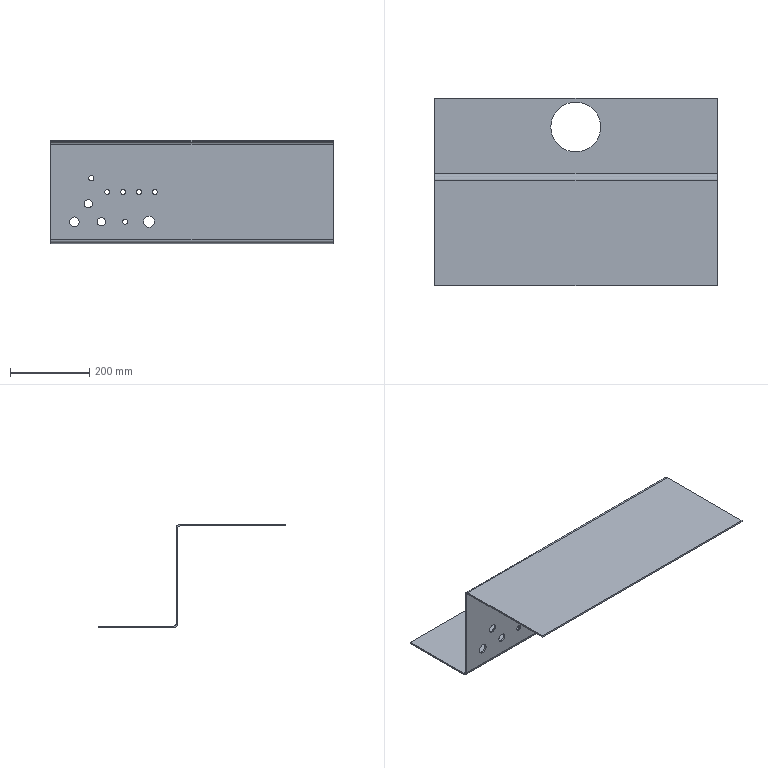Part | SolidWorks | features ICE 2, FlatPattern 1, SMBaseFlange 1, SheetMetal 1 | 1 solid | 44 faces | box 711 x 472 x 260 mm | volume 1991035 mm3 | cylinder 26 | plane 18 | commonest cylinder face diameters 12.5 x10 20.5 x4 12 x2 13.2 x2 20 x2 24.5 x2
STEP:
#1=CARTESIAN_POINT('',(-296.5,-200.,38.75));
#2=VERTEX_POINT('',#1);
#3=CARTESIAN_POINT('',(-296.5,-200.,63.25));
#4=VERTEX_POINT('',#3);
#5=CARTESIAN_POINT('',(-296.5,-200.,51.));
#6=DIRECTION('',(0.,1.,0.));
#7=DIRECTION('',(0.,0.,-1.));
#8=AXIS2_PLACEMENT_3D('',#5,#6,#7);
#9=CIRCLE('',#8,12.25);
#10=EDGE_CURVE('',#2,#4,#9,.T.);
#11=ORIENTED_EDGE('',*,*,#10,.F.);
#12=CARTESIAN_POINT('',(-296.5,-196.,38.75));
#13=VERTEX_POINT('',#12);
#14=CARTESIAN_POINT('',(-296.5,-472.001,38.75));
#15=DIRECTION('',(0.,1.,0.));
#16=VECTOR('',#15,1000.);
#17=LINE('',#14,#16);
#18=EDGE_CURVE('',#2,#13,#17,.T.);
#19=ORIENTED_EDGE('',*,*,#18,.T.);
#20=CARTESIAN_POINT('',(-296.5,-196.,63.25));
#21=VERTEX_POINT('',#20);
#22=CARTESIAN_POINT('',(-296.5,-196.,51.));
#23=DIRECTION('',(0.,1.,0.));
#24=DIRECTION('',(0.,0.,1.));
#25=AXIS2_PLACEMENT_3D('',#22,#23,#24);
#26=CIRCLE('',#25,12.25);
#27=EDGE_CURVE('',#13,#21,#26,.T.);
#28=ORIENTED_EDGE('',*,*,#27,.T.);
#29=CARTESIAN_POINT('',(-296.5,-472.001,63.25));
#30=DIRECTION('',(0.,1.,0.));
#31=VECTOR('',#30,1000.);
#32=LINE('',#29,#31);
#33=EDGE_CURVE('',#4,#21,#32,.T.);
#34=ORIENTED_EDGE('',*,*,#33,.F.);
#35=EDGE_LOOP('',(#11,#19,#28,#34));
#36=FACE_OUTER_BOUND('',#35,.T.);
#37=CARTESIAN_POINT('',(-296.5,-472.001,51.));
#38=DIRECTION('',(0.,1.,0.));
#39=DIRECTION('',(0.,0.,1.));
#40=AXIS2_PLACEMENT_3D('',#37,#38,#39);
#41=CYLINDRICAL_SURFACE('',#40,12.25);
#42=ADVANCED_FACE('',(#36),#41,.F.);
#43=CARTESIAN_POINT('',(-261.5,-200.,85.75));
#44=VERTEX_POINT('',#43);
#45=CARTESIAN_POINT('',(-261.5,-200.,106.25));
#46=VERTEX_POINT('',#45);
#47=CARTESIAN_POINT('',(-261.5,-200.,96.));
#48=DIRECTION('',(0.,1.,0.));
#49=DIRECTION('',(0.,0.,-1.));
#50=AXIS2_PLACEMENT_3D('',#47,#48,#49);
#51=CIRCLE('',#50,10.25);
#52=EDGE_CURVE('',#44,#46,#51,.T.);
#53=ORIENTED_EDGE('',*,*,#52,.F.);
#54=CARTESIAN_POINT('',(-261.5,-196.,85.75));
#55=VERTEX_POINT('',#54);
#56=CARTESIAN_POINT('',(-261.5,-472.001,85.75));
#57=DIRECTION('',(0.,1.,0.));
#58=VECTOR('',#57,1000.);
#59=LINE('',#56,#58);
#60=EDGE_CURVE('',#44,#55,#59,.T.);
#61=ORIENTED_EDGE('',*,*,#60,.T.);
#62=CARTESIAN_POINT('',(-261.5,-196.,106.25));
#63=VERTEX_POINT('',#62);
#64=CARTESIAN_POINT('',(-261.5,-196.,96.));
#65=DIRECTION('',(0.,1.,0.));
#66=DIRECTION('',(0.,0.,1.));
#67=AXIS2_PLACEMENT_3D('',#64,#65,#66);
#68=CIRCLE('',#67,10.25);
#69=EDGE_CURVE('',#55,#63,#68,.T.);
#70=ORIENTED_EDGE('',*,*,#69,.T.);
#71=CARTESIAN_POINT('',(-261.5,-472.001,106.25));
#72=DIRECTION('',(0.,1.,0.));
#73=VECTOR('',#72,1000.);
#74=LINE('',#71,#73);
#75=EDGE_CURVE('',#46,#63,#74,.T.);
#76=ORIENTED_EDGE('',*,*,#75,.F.);
#77=EDGE_LOOP('',(#53,#61,#70,#76));
#78=FACE_OUTER_BOUND('',#77,.T.);
#79=CARTESIAN_POINT('',(-261.5,-472.001,96.));
#80=DIRECTION('',(0.,1.,0.));
#81=DIRECTION('',(0.,0.,1.));
#82=AXIS2_PLACEMENT_3D('',#79,#80,#81);
#83=CYLINDRICAL_SURFACE('',#82,10.25);
#84=ADVANCED_FACE('',(#78),#83,.F.);
#85=CARTESIAN_POINT('',(-108.5,-200.,37.));
#86=VERTEX_POINT('',#85);
#87=CARTESIAN_POINT('',(-108.5,-200.,65.));
#88=VERTEX_POINT('',#87);
#89=CARTESIAN_POINT('',(-108.5,-200.,51.));
#90=DIRECTION('',(0.,1.,0.));
#91=DIRECTION('',(0.,0.,-1.));
#92=AXIS2_PLACEMENT_3D('',#89,#90,#91);
#93=CIRCLE('',#92,14.);
#94=EDGE_CURVE('',#86,#88,#93,.T.);
#95=ORIENTED_EDGE('',*,*,#94,.F.);
#96=CARTESIAN_POINT('',(-108.5,-196.,37.));
#97=VERTEX_POINT('',#96);
#98=CARTESIAN_POINT('',(-108.5,-472.001,37.));
#99=DIRECTION('',(0.,1.,0.));
#100=VECTOR('',#99,1000.);
#101=LINE('',#98,#100);
#102=EDGE_CURVE('',#86,#97,#101,.T.);
#103=ORIENTED_EDGE('',*,*,#102,.T.);
#104=CARTESIAN_POINT('',(-108.5,-196.,65.));
#105=VERTEX_POINT('',#104);
#106=CARTESIAN_POINT('',(-108.5,-196.,51.));
#107=DIRECTION('',(0.,1.,0.));
#108=DIRECTION('',(0.,0.,1.));
#109=AXIS2_PLACEMENT_3D('',#106,#107,#108);
#110=CIRCLE('',#109,14.);
#111=EDGE_CURVE('',#97,#105,#110,.T.);
#112=ORIENTED_EDGE('',*,*,#111,.T.);
#113=CARTESIAN_POINT('',(-108.5,-472.001,65.));
#114=DIRECTION('',(0.,1.,0.));
#115=VECTOR('',#114,1000.);
#116=LINE('',#113,#115);
#117=EDGE_CURVE('',#88,#105,#116,.T.);
#118=ORIENTED_EDGE('',*,*,#117,.F.);
#119=EDGE_LOOP('',(#95,#103,#112,#118));
#120=FACE_OUTER_BOUND('',#119,.T.);
#121=CARTESIAN_POINT('',(-108.5,-472.001,51.));
#122=DIRECTION('',(0.,1.,0.));
#123=DIRECTION('',(0.,0.,1.));
#124=AXIS2_PLACEMENT_3D('',#121,#122,#123);
#125=CYLINDRICAL_SURFACE('',#124,14.);
#126=ADVANCED_FACE('',(#120),#125,.F.);
#127=CARTESIAN_POINT('',(-168.5,-200.,44.75));
#128=VERTEX_POINT('',#127);
#129=CARTESIAN_POINT('',(-168.5,-200.,57.25));
#130=VERTEX_POINT('',#129);
#131=CARTESIAN_POINT('',(-168.5,-200.,51.));
#132=DIRECTION('',(0.,1.,0.));
#133=DIRECTION('',(0.,0.,-1.));
#134=AXIS2_PLACEMENT_3D('',#131,#132,#133);
#135=CIRCLE('',#134,6.25);
#136=EDGE_CURVE('',#128,#130,#135,.T.);
#137=ORIENTED_EDGE('',*,*,#136,.F.);
#138=CARTESIAN_POINT('',(-168.5,-196.,44.75));
#139=VERTEX_POINT('',#138);
#140=CARTESIAN_POINT('',(-168.5,-472.001,44.75));
#141=DIRECTION('',(0.,1.,0.));
#142=VECTOR('',#141,1000.);
#143=LINE('',#140,#142);
#144=EDGE_CURVE('',#128,#139,#143,.T.);
#145=ORIENTED_EDGE('',*,*,#144,.T.);
#146=CARTESIAN_POINT('',(-168.5,-196.,57.25));
#147=VERTEX_POINT('',#146);
#148=CARTESIAN_POINT('',(-168.5,-196.,51.));
#149=DIRECTION('',(0.,1.,0.));
#150=DIRECTION('',(0.,0.,1.));
#151=AXIS2_PLACEMENT_3D('',#148,#149,#150);
#152=CIRCLE('',#151,6.25);
#153=EDGE_CURVE('',#139,#147,#152,.T.);
#154=ORIENTED_EDGE('',*,*,#153,.T.);
#155=CARTESIAN_POINT('',(-168.5,-472.001,57.25));
#156=DIRECTION('',(0.,1.,0.));
#157=VECTOR('',#156,1000.);
#158=LINE('',#155,#157);
#159=EDGE_CURVE('',#130,#147,#158,.T.);
#160=ORIENTED_EDGE('',*,*,#159,.F.);
#161=EDGE_LOOP('',(#137,#145,#154,#160));
#162=FACE_OUTER_BOUND('',#161,.T.);
#163=CARTESIAN_POINT('',(-168.5,-472.001,51.));
#164=DIRECTION('',(0.,1.,0.));
#165=DIRECTION('',(0.,0.,1.));
#166=AXIS2_PLACEMENT_3D('',#163,#164,#165);
#167=CYLINDRICAL_SURFACE('',#166,6.25);
#168=ADVANCED_FACE('',(#162),#167,.F.);
#169=CARTESIAN_POINT('',(-228.5,-200.,40.75));
#170=VERTEX_POINT('',#169);
#171=CARTESIAN_POINT('',(-228.5,-200.,61.25));
#172=VERTEX_POINT('',#171);
#173=CARTESIAN_POINT('',(-228.5,-200.,51.));
#174=DIRECTION('',(0.,1.,0.));
#175=DIRECTION('',(0.,0.,-1.));
#176=AXIS2_PLACEMENT_3D('',#173,#174,#175);
#177=CIRCLE('',#176,10.25);
#178=EDGE_CURVE('',#170,#172,#177,.T.);
#179=ORIENTED_EDGE('',*,*,#178,.F.);
#180=CARTESIAN_POINT('',(-228.5,-196.,40.75));
#181=VERTEX_POINT('',#180);
#182=CARTESIAN_POINT('',(-228.5,-472.001,40.75));
#183=DIRECTION('',(0.,1.,0.));
#184=VECTOR('',#183,1000.);
#185=LINE('',#182,#184);
#186=EDGE_CURVE('',#170,#181,#185,.T.);
#187=ORIENTED_EDGE('',*,*,#186,.T.);
#188=CARTESIAN_POINT('',(-228.5,-196.,61.25));
#189=VERTEX_POINT('',#188);
#190=CARTESIAN_POINT('',(-228.5,-196.,51.));
#191=DIRECTION('',(0.,1.,0.));
#192=DIRECTION('',(0.,0.,1.));
#193=AXIS2_PLACEMENT_3D('',#190,#191,#192);
#194=CIRCLE('',#193,10.25);
#195=EDGE_CURVE('',#181,#189,#194,.T.);
#196=ORIENTED_EDGE('',*,*,#195,.T.);
#197=CARTESIAN_POINT('',(-228.5,-472.001,61.25));
#198=DIRECTION('',(0.,1.,0.));
#199=VECTOR('',#198,1000.);
#200=LINE('',#197,#199);
#201=EDGE_CURVE('',#172,#189,#200,.T.);
#202=ORIENTED_EDGE('',*,*,#201,.F.);
#203=EDGE_LOOP('',(#179,#187,#196,#202));
#204=FACE_OUTER_BOUND('',#203,.T.);
#205=CARTESIAN_POINT('',(-228.5,-472.001,51.));
#206=DIRECTION('',(0.,1.,0.));
#207=DIRECTION('',(0.,0.,1.));
#208=AXIS2_PLACEMENT_3D('',#205,#206,#207);
#209=CYLINDRICAL_SURFACE('',#208,10.25);
#210=ADVANCED_FACE('',(#204),#209,.F.);
#211=CARTESIAN_POINT('',(-213.5,-200.,119.75));
#212=VERTEX_POINT('',#211);
#213=CARTESIAN_POINT('',(-213.5,-200.,132.25));
#214=VERTEX_POINT('',#213);
#215=CARTESIAN_POINT('',(-213.5,-200.,126.));
#216=DIRECTION('',(0.,1.,0.));
#217=DIRECTION('',(0.,0.,-1.));
#218=AXIS2_PLACEMENT_3D('',#215,#216,#217);
#219=CIRCLE('',#218,6.25);
#220=EDGE_CURVE('',#212,#214,#219,.T.);
#221=ORIENTED_EDGE('',*,*,#220,.F.);
#222=CARTESIAN_POINT('',(-213.5,-196.,119.75));
#223=VERTEX_POINT('',#222);
#224=CARTESIAN_POINT('',(-213.5,-472.001,119.75));
#225=DIRECTION('',(0.,1.,0.));
#226=VECTOR('',#225,1000.);
#227=LINE('',#224,#226);
#228=EDGE_CURVE('',#212,#223,#227,.T.);
#229=ORIENTED_EDGE('',*,*,#228,.T.);
#230=CARTESIAN_POINT('',(-213.5,-196.,132.25));
#231=VERTEX_POINT('',#230);
#232=CARTESIAN_POINT('',(-213.5,-196.,126.));
#233=DIRECTION('',(0.,1.,0.));
#234=DIRECTION('',(0.,0.,1.));
#235=AXIS2_PLACEMENT_3D('',#232,#233,#234);
#236=CIRCLE('',#235,6.25);
#237=EDGE_CURVE('',#223,#231,#236,.T.);
#238=ORIENTED_EDGE('',*,*,#237,.T.);
#239=CARTESIAN_POINT('',(-213.5,-472.001,132.25));
#240=DIRECTION('',(0.,1.,0.));
#241=VECTOR('',#240,1000.);
#242=LINE('',#239,#241);
#243=EDGE_CURVE('',#214,#231,#242,.T.);
#244=ORIENTED_EDGE('',*,*,#243,.F.);
#245=EDGE_LOOP('',(#221,#229,#238,#244));
#246=FACE_OUTER_BOUND('',#245,.T.);
#247=CARTESIAN_POINT('',(-213.5,-472.001,126.));
#248=DIRECTION('',(0.,1.,0.));
#249=DIRECTION('',(0.,0.,1.));
#250=AXIS2_PLACEMENT_3D('',#247,#248,#249);
#251=CYLINDRICAL_SURFACE('',#250,6.25);
#252=ADVANCED_FACE('',(#246),#251,.F.);
#253=CARTESIAN_POINT('',(-173.5,-200.,119.75));
#254=VERTEX_POINT('',#253);
#255=CARTESIAN_POINT('',(-173.5,-200.,132.25));
#256=VERTEX_POINT('',#255);
#257=CARTESIAN_POINT('',(-173.5,-200.,126.));
#258=DIRECTION('',(0.,1.,0.));
#259=DIRECTION('',(0.,0.,-1.));
#260=AXIS2_PLACEMENT_3D('',#257,#258,#259);
#261=CIRCLE('',#260,6.25);
#262=EDGE_CURVE('',#254,#256,#261,.T.);
#263=ORIENTED_EDGE('',*,*,#262,.F.);
#264=CARTESIAN_POINT('',(-173.5,-196.,119.75));
#265=VERTEX_POINT('',#264);
#266=CARTESIAN_POINT('',(-173.5,-472.001,119.75));
#267=DIRECTION('',(0.,1.,0.));
#268=VECTOR('',#267,1000.);
#269=LINE('',#266,#268);
#270=EDGE_CURVE('',#254,#265,#269,.T.);
#271=ORIENTED_EDGE('',*,*,#270,.T.);
#272=CARTESIAN_POINT('',(-173.5,-196.,132.25));
#273=VERTEX_POINT('',#272);
#274=CARTESIAN_POINT('',(-173.5,-196.,126.));
#275=DIRECTION('',(0.,1.,0.));
#276=DIRECTION('',(0.,0.,1.));
#277=AXIS2_PLACEMENT_3D('',#274,#275,#276);
#278=CIRCLE('',#277,6.25);
#279=EDGE_CURVE('',#265,#273,#278,.T.);
#280=ORIENTED_EDGE('',*,*,#279,.T.);
#281=CARTESIAN_POINT('',(-173.5,-472.001,132.25));
#282=DIRECTION('',(0.,1.,0.));
#283=VECTOR('',#282,1000.);
#284=LINE('',#281,#283);
#285=EDGE_CURVE('',#256,#273,#284,.T.);
#286=ORIENTED_EDGE('',*,*,#285,.F.);
#287=EDGE_LOOP('',(#263,#271,#280,#286));
#288=FACE_OUTER_BOUND('',#287,.T.);
#289=CARTESIAN_POINT('',(-173.5,-472.001,126.));
#290=DIRECTION('',(0.,1.,0.));
#291=DIRECTION('',(0.,0.,1.));
#292=AXIS2_PLACEMENT_3D('',#289,#290,#291);
#293=CYLINDRICAL_SURFACE('',#292,6.25);
#294=ADVANCED_FACE('',(#288),#293,.F.);
#295=CARTESIAN_POINT('',(-133.5,-200.,119.75));
#296=VERTEX_POINT('',#295);
#297=CARTESIAN_POINT('',(-133.5,-200.,132.25));
#298=VERTEX_POINT('',#297);
#299=CARTESIAN_POINT('',(-133.5,-200.,126.));
#300=DIRECTION('',(0.,1.,0.));
#301=DIRECTION('',(0.,0.,-1.));
#302=AXIS2_PLACEMENT_3D('',#299,#300,#301);
#303=CIRCLE('',#302,6.25);
#304=EDGE_CURVE('',#296,#298,#303,.T.);
#305=ORIENTED_EDGE('',*,*,#304,.F.);
#306=CARTESIAN_POINT('',(-133.5,-196.,119.75));
#307=VERTEX_POINT('',#306);
#308=CARTESIAN_POINT('',(-133.5,-472.001,119.75));
#309=DIRECTION('',(0.,1.,0.));
#310=VECTOR('',#309,1000.);
#311=LINE('',#308,#310);
#312=EDGE_CURVE('',#296,#307,#311,.T.);
#313=ORIENTED_EDGE('',*,*,#312,.T.);
#314=CARTESIAN_POINT('',(-133.5,-196.,132.25));
#315=VERTEX_POINT('',#314);
#316=CARTESIAN_POINT('',(-133.5,-196.,126.));
#317=DIRECTION('',(0.,1.,0.));
#318=DIRECTION('',(0.,0.,1.));
#319=AXIS2_PLACEMENT_3D('',#316,#317,#318);
#320=CIRCLE('',#319,6.25);
#321=EDGE_CURVE('',#307,#315,#320,.T.);
#322=ORIENTED_EDGE('',*,*,#321,.T.);
#323=CARTESIAN_POINT('',(-133.5,-472.001,132.25));
#324=DIRECTION('',(0.,1.,0.));
#325=VECTOR('',#324,1000.);
#326=LINE('',#323,#325);
#327=EDGE_CURVE('',#298,#315,#326,.T.);
#328=ORIENTED_EDGE('',*,*,#327,.F.);
#329=EDGE_LOOP('',(#305,#313,#322,#328));
#330=FACE_OUTER_BOUND('',#329,.T.);
#331=CARTESIAN_POINT('',(-133.5,-472.001,126.));
#332=DIRECTION('',(0.,1.,0.));
#333=DIRECTION('',(0.,0.,1.));
#334=AXIS2_PLACEMENT_3D('',#331,#332,#333);
#335=CYLINDRICAL_SURFACE('',#334,6.25);
#336=ADVANCED_FACE('',(#330),#335,.F.);
#337=CARTESIAN_POINT('',(-93.5,-200.,119.75));
#338=VERTEX_POINT('',#337);
#339=CARTESIAN_POINT('',(-93.5,-200.,132.25));
#340=VERTEX_POINT('',#339);
#341=CARTESIAN_POINT('',(-93.5,-200.,126.));
#342=DIRECTION('',(0.,1.,0.));
#343=DIRECTION('',(0.,0.,-1.));
#344=AXIS2_PLACEMENT_3D('',#341,#342,#343);
#345=CIRCLE('',#344,6.25);
#346=EDGE_CURVE('',#338,#340,#345,.T.);
#347=ORIENTED_EDGE('',*,*,#346,.F.);
#348=CARTESIAN_POINT('',(-93.5,-196.,119.75));
#349=VERTEX_POINT('',#348);
#350=CARTESIAN_POINT('',(-93.5,-472.001,119.75));
#351=DIRECTION('',(0.,1.,0.));
#352=VECTOR('',#351,1000.);
#353=LINE('',#350,#352);
#354=EDGE_CURVE('',#338,#349,#353,.T.);
#355=ORIENTED_EDGE('',*,*,#354,.T.);
#356=CARTESIAN_POINT('',(-93.5,-196.,132.25));
#357=VERTEX_POINT('',#356);
#358=CARTESIAN_POINT('',(-93.5,-196.,126.));
#359=DIRECTION('',(0.,1.,0.));
#360=DIRECTION('',(0.,0.,1.));
#361=AXIS2_PLACEMENT_3D('',#358,#359,#360);
#362=CIRCLE('',#361,6.25);
#363=EDGE_CURVE('',#349,#357,#362,.T.);
#364=ORIENTED_EDGE('',*,*,#363,.T.);
#365=CARTESIAN_POINT('',(-93.5,-472.001,132.25));
#366=DIRECTION('',(0.,1.,0.));
#367=VECTOR('',#366,1000.);
#368=LINE('',#365,#367);
#369=EDGE_CURVE('',#340,#357,#368,.T.);
#370=ORIENTED_EDGE('',*,*,#369,.F.);
#371=EDGE_LOOP('',(#347,#355,#364,#370));
#372=FACE_OUTER_BOUND('',#371,.T.);
#373=CARTESIAN_POINT('',(-93.5,-472.001,126.));
#374=DIRECTION('',(0.,1.,0.));
#375=DIRECTION('',(0.,0.,1.));
#376=AXIS2_PLACEMENT_3D('',#373,#374,#375);
#377=CYLINDRICAL_SURFACE('',#376,6.25);
#378=ADVANCED_FACE('',(#372),#377,.F.);
#379=CARTESIAN_POINT('',(-253.5,-200.,154.4));
#380=VERTEX_POINT('',#379);
#381=CARTESIAN_POINT('',(-253.5,-200.,167.6));
#382=VERTEX_POINT('',#381);
#383=CARTESIAN_POINT('',(-253.5,-200.,161.));
#384=DIRECTION('',(0.,1.,0.));
#385=DIRECTION('',(0.,0.,-1.));
#386=AXIS2_PLACEMENT_3D('',#383,#384,#385);
#387=CIRCLE('',#386,6.6);
#388=EDGE_CURVE('',#380,#382,#387,.T.);
#389=ORIENTED_EDGE('',*,*,#388,.F.);
#390=CARTESIAN_POINT('',(-253.5,-196.,154.4));
#391=VERTEX_POINT('',#390);
#392=CARTESIAN_POINT('',(-253.5,-472.001,154.4));
#393=DIRECTION('',(0.,1.,0.));
#394=VECTOR('',#393,1000.);
#395=LINE('',#392,#394);
#396=EDGE_CURVE('',#380,#391,#395,.T.);
#397=ORIENTED_EDGE('',*,*,#396,.T.);
#398=CARTESIAN_POINT('',(-253.5,-196.,167.6));
#399=VERTEX_POINT('',#398);
#400=CARTESIAN_POINT('',(-253.5,-196.,161.));
#401=DIRECTION('',(0.,1.,0.));
#402=DIRECTION('',(0.,0.,1.));
#403=AXIS2_PLACEMENT_3D('',#400,#401,#402);
#404=CIRCLE('',#403,6.6);
#405=EDGE_CURVE('',#391,#399,#404,.T.);
#406=ORIENTED_EDGE('',*,*,#405,.T.);
#407=CARTESIAN_POINT('',(-253.5,-472.001,167.6));
#408=DIRECTION('',(0.,1.,0.));
#409=VECTOR('',#408,1000.);
#410=LINE('',#407,#409);
#411=EDGE_CURVE('',#382,#399,#410,.T.);
#412=ORIENTED_EDGE('',*,*,#411,.F.);
#413=EDGE_LOOP('',(#389,#397,#406,#412));
#414=FACE_OUTER_BOUND('',#413,.T.);
#415=CARTESIAN_POINT('',(-253.5,-472.001,161.));
#416=DIRECTION('',(0.,1.,0.));
#417=DIRECTION('',(0.,0.,1.));
#418=AXIS2_PLACEMENT_3D('',#415,#416,#417);
#419=CYLINDRICAL_SURFACE('',#418,6.6);
#420=ADVANCED_FACE('',(#414),#419,.F.);
#421=CARTESIAN_POINT('',(-63.7,-72.,0.));
#422=VERTEX_POINT('',#421);
#423=CARTESIAN_POINT('',(62.3,-72.,0.));
#424=VERTEX_POINT('',#423);
#425=CARTESIAN_POINT('',(-0.7,-72.,0.));
#426=DIRECTION('',(0.,0.,1.));
#427=DIRECTION('',(-1.,0.,0.));
#428=AXIS2_PLACEMENT_3D('',#425,#426,#427);
#429=CIRCLE('',#428,63.);
#430=EDGE_CURVE('',#422,#424,#429,.T.);
#431=ORIENTED_EDGE('',*,*,#430,.T.);
#432=CARTESIAN_POINT('',(62.3,-72.,-4.));
#433=VERTEX_POINT('',#432);
#434=CARTESIAN_POINT('',(62.3,-72.,256.001));
#435=DIRECTION('',(0.,0.,-1.));
#436=VECTOR('',#435,1000.);
#437=LINE('',#434,#436);
#438=EDGE_CURVE('',#424,#433,#437,.T.);
#439=ORIENTED_EDGE('',*,*,#438,.T.);
#440=CARTESIAN_POINT('',(-63.7,-72.,-4.));
#441=VERTEX_POINT('',#440);
#442=CARTESIAN_POINT('',(-0.7,-72.,-4.));
#443=DIRECTION('',(0.,0.,-1.));
#444=DIRECTION('',(-1.,0.,0.));
#445=AXIS2_PLACEMENT_3D('',#442,#443,#444);
#446=CIRCLE('',#445,63.);
#447=EDGE_CURVE('',#433,#441,#446,.T.);
#448=ORIENTED_EDGE('',*,*,#447,.T.);
#449=CARTESIAN_POINT('',(-63.7,-72.,256.001));
#450=DIRECTION('',(0.,0.,-1.));
#451=VECTOR('',#450,1000.);
#452=LINE('',#449,#451);
#453=EDGE_CURVE('',#422,#441,#452,.T.);
#454=ORIENTED_EDGE('',*,*,#453,.F.);
#455=EDGE_LOOP('',(#431,#439,#448,#454));
#456=FACE_OUTER_BOUND('',#455,.T.);
#457=CARTESIAN_POINT('',(-0.7,-72.,256.001));
#458=DIRECTION('',(0.,0.,-1.));
#459=DIRECTION('',(-1.,0.,0.));
#460=AXIS2_PLACEMENT_3D('',#457,#458,#459);
#461=CYLINDRICAL_SURFACE('',#460,63.);
#462=ADVANCED_FACE('',(#456),#461,.F.);
#463=CARTESIAN_POINT('',(355.5,-190.,0.));
#464=VERTEX_POINT('',#463);
#465=CARTESIAN_POINT('',(355.5,-190.,-4.));
#466=VERTEX_POINT('',#465);
#467=CARTESIAN_POINT('',(355.5,-190.,0.));
#468=DIRECTION('',(0.,0.,-1.));
#469=VECTOR('',#468,1000.);
#470=LINE('',#467,#469);
#471=EDGE_CURVE('',#464,#466,#470,.T.);
#472=ORIENTED_EDGE('',*,*,#471,.F.);
#473=CARTESIAN_POINT('',(355.5,-196.,6.));
#474=VERTEX_POINT('',#473);
#475=CARTESIAN_POINT('',(355.5,-190.,6.));
#476=DIRECTION('',(-1.,0.,0.));
#477=DIRECTION('',(0.,0.,-1.));
#478=AXIS2_PLACEMENT_3D('',#475,#476,#477);
#479=CIRCLE('',#478,6.);
#480=EDGE_CURVE('',#464,#474,#479,.T.);
#481=ORIENTED_EDGE('',*,*,#480,.T.);
#482=CARTESIAN_POINT('',(355.5,-200.,6.));
#483=VERTEX_POINT('',#482);
#484=CARTESIAN_POINT('',(355.5,-200.,6.));
#485=DIRECTION('',(0.,1.,0.));
#486=VECTOR('',#485,1000.);
#487=LINE('',#484,#486);
#488=EDGE_CURVE('',#483,#474,#487,.T.);
#489=ORIENTED_EDGE('',*,*,#488,.F.);
#490=CARTESIAN_POINT('',(355.5,-190.,6.));
#491=DIRECTION('',(-1.,0.,0.));
#492=DIRECTION('',(0.,0.,-1.));
#493=AXIS2_PLACEMENT_3D('',#490,#491,#492);
#494=CIRCLE('',#493,10.);
#495=EDGE_CURVE('',#466,#483,#494,.T.);
#496=ORIENTED_EDGE('',*,*,#495,.F.);
#497=EDGE_LOOP('',(#472,#481,#489,#496));
#498=FACE_OUTER_BOUND('',#497,.T.);
#499=CARTESIAN_POINT('',(355.5,-190.,0.));
#500=DIRECTION('',(1.,0.,0.));
#501=DIRECTION('',(0.,0.,-1.));
#502=AXIS2_PLACEMENT_3D('',#499,#500,#501);
#503=PLANE('',#502);
#504=ADVANCED_FACE('',(#498),#503,.T.);
#505=CARTESIAN_POINT('',(355.5,0.,0.));
#506=VERTEX_POINT('',#505);
#507=CARTESIAN_POINT('',(355.5,0.,0.));
#508=DIRECTION('',(0.,-1.,0.));
#509=VECTOR('',#508,1000.);
#510=LINE('',#507,#509);
#511=EDGE_CURVE('',#506,#464,#510,.T.);
#512=ORIENTED_EDGE('',*,*,#511,.T.);
#513=ORIENTED_EDGE('',*,*,#471,.T.);
#514=CARTESIAN_POINT('',(355.5,0.,-4.));
#515=VERTEX_POINT('',#514);
#516=CARTESIAN_POINT('',(355.5,0.,-4.));
#517=DIRECTION('',(0.,-1.,0.));
#518=VECTOR('',#517,1000.);
#519=LINE('',#516,#518);
#520=EDGE_CURVE('',#515,#466,#519,.T.);
#521=ORIENTED_EDGE('',*,*,#520,.F.);
#522=CARTESIAN_POINT('',(355.5,0.,0.));
#523=DIRECTION('',(0.,0.,-1.));
#524=VECTOR('',#523,1000.);
#525=LINE('',#522,#524);
#526=EDGE_CURVE('',#506,#515,#525,.T.);
#527=ORIENTED_EDGE('',*,*,#526,.F.);
#528=EDGE_LOOP('',(#512,#513,#521,#527));
#529=FACE_OUTER_BOUND('',#528,.T.);
#530=CARTESIAN_POINT('',(355.5,-200.,6.));
#531=DIRECTION('',(1.,0.,0.));
#532=DIRECTION('',(0.,0.,-1.));
#533=AXIS2_PLACEMENT_3D('',#530,#531,#532);
#534=PLANE('',#533);
#535=ADVANCED_FACE('',(#529),#534,.T.);
#536=CARTESIAN_POINT('',(-355.5,-196.,6.));
#537=VERTEX_POINT('',#536);
#538=CARTESIAN_POINT('',(-355.5,-200.,6.));
#539=VERTEX_POINT('',#538);
#540=CARTESIAN_POINT('',(-355.5,-196.,6.));
#541=DIRECTION('',(0.,-1.,0.));
#542=VECTOR('',#541,1000.);
#543=LINE('',#540,#542);
#544=EDGE_CURVE('',#537,#539,#543,.T.);
#545=ORIENTED_EDGE('',*,*,#544,.F.);
#546=CARTESIAN_POINT('',(-355.5,-190.,0.));
#547=VERTEX_POINT('',#546);
#548=CARTESIAN_POINT('',(-355.5,-190.,6.));
#549=DIRECTION('',(-1.,0.,0.));
#550=DIRECTION('',(0.,0.,-1.));
#551=AXIS2_PLACEMENT_3D('',#548,#549,#550);
#552=CIRCLE('',#551,6.);
#553=EDGE_CURVE('',#547,#537,#552,.T.);
#554=ORIENTED_EDGE('',*,*,#553,.F.);
#555=CARTESIAN_POINT('',(-355.5,-190.,-4.));
#556=VERTEX_POINT('',#555);
#557=CARTESIAN_POINT('',(-355.5,-190.,-4.));
#558=DIRECTION('',(0.,0.,1.));
#559=VECTOR('',#558,1000.);
#560=LINE('',#557,#559);
#561=EDGE_CURVE('',#556,#547,#560,.T.);
#562=ORIENTED_EDGE('',*,*,#561,.F.);
#563=CARTESIAN_POINT('',(-355.5,-190.,6.));
#564=DIRECTION('',(-1.,0.,0.));
#565=DIRECTION('',(0.,0.,-1.));
#566=AXIS2_PLACEMENT_3D('',#563,#564,#565);
#567=CIRCLE('',#566,10.);
#568=EDGE_CURVE('',#556,#539,#567,.T.);
#569=ORIENTED_EDGE('',*,*,#568,.T.);
#570=EDGE_LOOP('',(#545,#554,#562,#569));
#571=FACE_OUTER_BOUND('',#570,.T.);
#572=CARTESIAN_POINT('',(-355.5,-196.,6.));
#573=DIRECTION('',(-1.,0.,0.));
#574=DIRECTION('',(0.,0.,1.));
#575=AXIS2_PLACEMENT_3D('',#572,#573,#574);
#576=PLANE('',#575);
#577=ADVANCED_FACE('',(#571),#576,.T.);
#578=CARTESIAN_POINT('',(-355.5,-196.,246.));
#579=VERTEX_POINT('',#578);
#580=CARTESIAN_POINT('',(-355.5,-196.,0.));
#581=DIRECTION('',(0.,0.,1.));
#582=VECTOR('',#581,1000.);
#583=LINE('',#580,#582);
#584=EDGE_CURVE('',#537,#579,#583,.T.);
#585=ORIENTED_EDGE('',*,*,#584,.F.);
#586=ORIENTED_EDGE('',*,*,#544,.T.);
#587=CARTESIAN_POINT('',(-355.5,-200.,246.));
#588=VERTEX_POINT('',#587);
#589=CARTESIAN_POINT('',(-355.5,-200.,0.));
#590=DIRECTION('',(0.,0.,1.));
#591=VECTOR('',#590,1000.);
#592=LINE('',#589,#591);
#593=EDGE_CURVE('',#539,#588,#592,.T.);
#594=ORIENTED_EDGE('',*,*,#593,.T.);
#595=CARTESIAN_POINT('',(-355.5,-200.,246.));
#596=DIRECTION('',(0.,1.,0.));
#597=VECTOR('',#596,1000.);
#598=LINE('',#595,#597);
#599=EDGE_CURVE('',#588,#579,#598,.T.);
#600=ORIENTED_EDGE('',*,*,#599,.T.);
#601=EDGE_LOOP('',(#585,#586,#594,#600));
#602=FACE_OUTER_BOUND('',#601,.T.);
#603=CARTESIAN_POINT('',(-355.5,-190.,-4.));
#604=DIRECTION('',(-1.,0.,0.));
#605=DIRECTION('',(0.,0.,1.));
#606=AXIS2_PLACEMENT_3D('',#603,#604,#605);
#607=PLANE('',#606);
#608=ADVANCED_FACE('',(#602),#607,.T.);
#609=CARTESIAN_POINT('',(355.5,-196.,246.));
#610=VERTEX_POINT('',#609);
#611=CARTESIAN_POINT('',(355.5,-200.,246.));
#612=VERTEX_POINT('',#611);
#613=CARTESIAN_POINT('',(355.5,-196.,246.));
#614=DIRECTION('',(0.,-1.,0.));
#615=VECTOR('',#614,1000.);
#616=LINE('',#613,#615);
#617=EDGE_CURVE('',#610,#612,#616,.T.);
#618=ORIENTED_EDGE('',*,*,#617,.F.);
#619=CARTESIAN_POINT('',(355.5,-206.,256.));
#620=VERTEX_POINT('',#619);
#621=CARTESIAN_POINT('',(355.5,-206.,246.));
#622=DIRECTION('',(1.,0.,0.));
#623=DIRECTION('',(0.,0.,1.));
#624=AXIS2_PLACEMENT_3D('',#621,#622,#623);
#625=CIRCLE('',#624,10.);
#626=EDGE_CURVE('',#610,#620,#625,.T.);
#627=ORIENTED_EDGE('',*,*,#626,.T.);
#628=CARTESIAN_POINT('',(355.5,-206.,252.));
#629=VERTEX_POINT('',#628);
#630=CARTESIAN_POINT('',(355.5,-206.,252.));
#631=DIRECTION('',(0.,0.,1.));
#632=VECTOR('',#631,1000.);
#633=LINE('',#630,#632);
#634=EDGE_CURVE('',#629,#620,#633,.T.);
#635=ORIENTED_EDGE('',*,*,#634,.F.);
#636=CARTESIAN_POINT('',(355.5,-206.,246.));
#637=DIRECTION('',(1.,0.,0.));
#638=DIRECTION('',(0.,0.,-1.));
#639=AXIS2_PLACEMENT_3D('',#636,#637,#638);
#640=CIRCLE('',#639,6.);
#641=EDGE_CURVE('',#612,#629,#640,.T.);
#642=ORIENTED_EDGE('',*,*,#641,.F.);
#643=EDGE_LOOP('',(#618,#627,#635,#642));
#644=FACE_OUTER_BOUND('',#643,.T.);
#645=CARTESIAN_POINT('',(355.5,-196.,246.));
#646=DIRECTION('',(1.,0.,0.));
#647=DIRECTION('',(0.,0.,-1.));
#648=AXIS2_PLACEMENT_3D('',#645,#646,#647);
#649=PLANE('',#648);
#650=ADVANCED_FACE('',(#644),#649,.T.);
#651=CARTESIAN_POINT('',(355.5,-196.,0.));
#652=DIRECTION('',(0.,0.,1.));
#653=VECTOR('',#652,1000.);
#654=LINE('',#651,#653);
#655=EDGE_CURVE('',#474,#610,#654,.T.);
#656=ORIENTED_EDGE('',*,*,#655,.T.);
#657=ORIENTED_EDGE('',*,*,#617,.T.);
#658=CARTESIAN_POINT('',(355.5,-200.,0.));
#659=DIRECTION('',(0.,0.,1.));
#660=VECTOR('',#659,1000.);
#661=LINE('',#658,#660);
#662=EDGE_CURVE('',#483,#612,#661,.T.);
#663=ORIENTED_EDGE('',*,*,#662,.F.);
#664=ORIENTED_EDGE('',*,*,#488,.T.);
#665=EDGE_LOOP('',(#656,#657,#663,#664));
#666=FACE_OUTER_BOUND('',#665,.T.);
#667=CARTESIAN_POINT('',(355.5,-206.,252.));
#668=DIRECTION('',(1.,0.,0.));
#669=DIRECTION('',(0.,0.,-1.));
#670=AXIS2_PLACEMENT_3D('',#667,#668,#669);
#671=PLANE('',#670);
#672=ADVANCED_FACE('',(#666),#671,.T.);
#673=CARTESIAN_POINT('',(-355.5,-206.,256.));
#674=VERTEX_POINT('',#673);
#675=CARTESIAN_POINT('',(-355.5,-206.,252.));
#676=VERTEX_POINT('',#675);
#677=CARTESIAN_POINT('',(-355.5,-206.,256.));
#678=DIRECTION('',(0.,0.,-1.));
#679=VECTOR('',#678,1000.);
#680=LINE('',#677,#679);
#681=EDGE_CURVE('',#674,#676,#680,.T.);
#682=ORIENTED_EDGE('',*,*,#681,.F.);
#683=CARTESIAN_POINT('',(-355.5,-206.,246.));
#684=DIRECTION('',(1.,0.,0.));
#685=DIRECTION('',(0.,0.,1.));
#686=AXIS2_PLACEMENT_3D('',#683,#684,#685);
#687=CIRCLE('',#686,10.);
#688=EDGE_CURVE('',#579,#674,#687,.T.);
#689=ORIENTED_EDGE('',*,*,#688,.F.);
#690=ORIENTED_EDGE('',*,*,#599,.F.);
#691=CARTESIAN_POINT('',(-355.5,-206.,246.));
#692=DIRECTION('',(1.,0.,0.));
#693=DIRECTION('',(0.,0.,-1.));
#694=AXIS2_PLACEMENT_3D('',#691,#692,#693);
#695=CIRCLE('',#694,6.);
#696=EDGE_CURVE('',#588,#676,#695,.T.);
#697=ORIENTED_EDGE('',*,*,#696,.T.);
#698=EDGE_LOOP('',(#682,#689,#690,#697));
#699=FACE_OUTER_BOUND('',#698,.T.);
#700=CARTESIAN_POINT('',(-355.5,-206.,256.));
#701=DIRECTION('',(-1.,0.,0.));
#702=DIRECTION('',(0.,0.,1.));
#703=AXIS2_PLACEMENT_3D('',#700,#701,#702);
#704=PLANE('',#703);
#705=ADVANCED_FACE('',(#699),#704,.T.);
#706=CARTESIAN_POINT('',(-355.5,-472.,256.));
#707=VERTEX_POINT('',#706);
#708=CARTESIAN_POINT('',(-355.5,-196.,256.));
#709=DIRECTION('',(0.,-1.,0.));
#710=VECTOR('',#709,1000.);
#711=LINE('',#708,#710);
#712=EDGE_CURVE('',#674,#707,#711,.T.);
#713=ORIENTED_EDGE('',*,*,#712,.F.);
#714=ORIENTED_EDGE('',*,*,#681,.T.);
#715=CARTESIAN_POINT('',(-355.5,-472.,252.));
#716=VERTEX_POINT('',#715);
#717=CARTESIAN_POINT('',(-355.5,-196.,252.));
#718=DIRECTION('',(0.,-1.,0.));
#719=VECTOR('',#718,1000.);
#720=LINE('',#717,#719);
#721=EDGE_CURVE('',#676,#716,#720,.T.);
#722=ORIENTED_EDGE('',*,*,#721,.T.);
#723=CARTESIAN_POINT('',(-355.5,-472.,252.));
#724=DIRECTION('',(0.,0.,1.));
#725=VECTOR('',#724,1000.);
#726=LINE('',#723,#725);
#727=EDGE_CURVE('',#716,#707,#726,.T.);
#728=ORIENTED_EDGE('',*,*,#727,.T.);
#729=EDGE_LOOP('',(#713,#714,#722,#728));
#730=FACE_OUTER_BOUND('',#729,.T.);
#731=CARTESIAN_POINT('',(-355.5,-200.,246.));
#732=DIRECTION('',(-1.,0.,0.));
#733=DIRECTION('',(0.,0.,1.));
#734=AXIS2_PLACEMENT_3D('',#731,#732,#733);
#735=PLANE('',#734);
#736=ADVANCED_FACE('',(#730),#735,.T.);
#737=ORIENTED_EDGE('',*,*,#712,.T.);
#738=CARTESIAN_POINT('',(355.5,-472.,256.));
#739=VERTEX_POINT('',#738);
#740=CARTESIAN_POINT('',(355.5,-472.,256.));
#741=DIRECTION('',(-1.,0.,0.));
#742=VECTOR('',#741,1000.);
#743=LINE('',#740,#742);
#744=EDGE_CURVE('',#739,#707,#743,.T.);
#745=ORIENTED_EDGE('',*,*,#744,.F.);
#746=CARTESIAN_POINT('',(355.5,-196.,256.));
#747=DIRECTION('',(0.,-1.,0.));
#748=VECTOR('',#747,1000.);
#749=LINE('',#746,#748);
#750=EDGE_CURVE('',#620,#739,#749,.T.);
#751=ORIENTED_EDGE('',*,*,#750,.F.);
#752=CARTESIAN_POINT('',(355.5,-206.,256.));
#753=DIRECTION('',(-1.,0.,0.));
#754=VECTOR('',#753,1000.);
#755=LINE('',#752,#754);
#756=EDGE_CURVE('',#620,#674,#755,.T.);
#757=ORIENTED_EDGE('',*,*,#756,.T.);
#758=EDGE_LOOP('',(#737,#745,#751,#757));
#759=FACE_OUTER_BOUND('',#758,.T.);
#760=CARTESIAN_POINT('',(355.5,-196.,256.));
#761=DIRECTION('',(0.,0.,-1.));
#762=DIRECTION('',(0.,1.,0.));
#763=AXIS2_PLACEMENT_3D('',#760,#761,#762);
#764=PLANE('',#763);
#765=ADVANCED_FACE('',(#759),#764,.F.);
#766=ORIENTED_EDGE('',*,*,#727,.F.);
#767=CARTESIAN_POINT('',(355.5,-472.,252.));
#768=VERTEX_POINT('',#767);
#769=CARTESIAN_POINT('',(355.5,-472.,252.));
#770=DIRECTION('',(-1.,0.,0.));
#771=VECTOR('',#770,1000.);
#772=LINE('',#769,#771);
#773=EDGE_CURVE('',#768,#716,#772,.T.);
#774=ORIENTED_EDGE('',*,*,#773,.F.);
#775=CARTESIAN_POINT('',(355.5,-472.,252.));
#776=DIRECTION('',(0.,0.,1.));
#777=VECTOR('',#776,1000.);
#778=LINE('',#775,#777);
#779=EDGE_CURVE('',#768,#739,#778,.T.);
#780=ORIENTED_EDGE('',*,*,#779,.T.);
#781=ORIENTED_EDGE('',*,*,#744,.T.);
#782=EDGE_LOOP('',(#766,#774,#780,#781));
#783=FACE_OUTER_BOUND('',#782,.T.);
#784=CARTESIAN_POINT('',(355.5,-472.,252.));
#785=DIRECTION('',(0.,-1.,0.));
#786=DIRECTION('',(0.,0.,-1.));
#787=AXIS2_PLACEMENT_3D('',#784,#785,#786);
#788=PLANE('',#787);
#789=ADVANCED_FACE('',(#783),#788,.T.);
#790=ORIENTED_EDGE('',*,*,#721,.F.);
#791=CARTESIAN_POINT('',(355.5,-206.,252.));
#792=DIRECTION('',(-1.,0.,0.));
#793=VECTOR('',#792,1000.);
#794=LINE('',#791,#793);
#795=EDGE_CURVE('',#629,#676,#794,.T.);
#796=ORIENTED_EDGE('',*,*,#795,.F.);
#797=CARTESIAN_POINT('',(355.5,-196.,252.));
#798=DIRECTION('',(0.,-1.,0.));
#799=VECTOR('',#798,1000.);
#800=LINE('',#797,#799);
#801=EDGE_CURVE('',#629,#768,#800,.T.);
#802=ORIENTED_EDGE('',*,*,#801,.T.);
#803=ORIENTED_EDGE('',*,*,#773,.T.);
#804=EDGE_LOOP('',(#790,#796,#802,#803));
#805=FACE_OUTER_BOUND('',#804,.T.);
#806=CARTESIAN_POINT('',(355.5,-196.,252.));
#807=DIRECTION('',(0.,0.,-1.));
#808=DIRECTION('',(0.,1.,0.));
#809=AXIS2_PLACEMENT_3D('',#806,#807,#808);
#810=PLANE('',#809);
#811=ADVANCED_FACE('',(#805),#810,.T.);
#812=ORIENTED_EDGE('',*,*,#696,.F.);
#813=CARTESIAN_POINT('',(355.5,-200.,246.));
#814=DIRECTION('',(-1.,0.,0.));
#815=VECTOR('',#814,1000.);
#816=LINE('',#813,#815);
#817=EDGE_CURVE('',#612,#588,#816,.T.);
#818=ORIENTED_EDGE('',*,*,#817,.F.);
#819=ORIENTED_EDGE('',*,*,#641,.T.);
#820=ORIENTED_EDGE('',*,*,#795,.T.);
#821=EDGE_LOOP('',(#812,#818,#819,#820));
#822=FACE_OUTER_BOUND('',#821,.T.);
#823=CARTESIAN_POINT('',(355.5,-206.,246.));
#824=DIRECTION('',(-1.,0.,0.));
#825=DIRECTION('',(0.,0.,1.));
#826=AXIS2_PLACEMENT_3D('',#823,#824,#825);
#827=CYLINDRICAL_SURFACE('',#826,6.);
#828=ADVANCED_FACE('',(#822),#827,.F.);
#829=CARTESIAN_POINT('',(-296.5,-200.,51.));
#830=DIRECTION('',(0.,1.,0.));
#831=DIRECTION('',(0.,0.,-1.));
#832=AXIS2_PLACEMENT_3D('',#829,#830,#831);
#833=CIRCLE('',#832,12.25);
#834=EDGE_CURVE('',#4,#2,#833,.T.);
#835=ORIENTED_EDGE('',*,*,#834,.T.);
#836=ORIENTED_EDGE('',*,*,#10,.T.);
#837=EDGE_LOOP('',(#835,#836));
#838=FACE_BOUND('',#837,.T.);
#839=CARTESIAN_POINT('',(-261.5,-200.,96.));
#840=DIRECTION('',(0.,1.,0.));
#841=DIRECTION('',(0.,0.,-1.));
#842=AXIS2_PLACEMENT_3D('',#839,#840,#841);
#843=CIRCLE('',#842,10.25);
#844=EDGE_CURVE('',#46,#44,#843,.T.);
#845=ORIENTED_EDGE('',*,*,#844,.T.);
#846=ORIENTED_EDGE('',*,*,#52,.T.);
#847=EDGE_LOOP('',(#845,#846));
#848=FACE_BOUND('',#847,.T.);
#849=CARTESIAN_POINT('',(-108.5,-200.,51.));
#850=DIRECTION('',(0.,1.,0.));
#851=DIRECTION('',(0.,0.,-1.));
#852=AXIS2_PLACEMENT_3D('',#849,#850,#851);
#853=CIRCLE('',#852,14.);
#854=EDGE_CURVE('',#88,#86,#853,.T.);
#855=ORIENTED_EDGE('',*,*,#854,.T.);
#856=ORIENTED_EDGE('',*,*,#94,.T.);
#857=EDGE_LOOP('',(#855,#856));
#858=FACE_BOUND('',#857,.T.);
#859=CARTESIAN_POINT('',(-168.5,-200.,51.));
#860=DIRECTION('',(0.,1.,0.));
#861=DIRECTION('',(0.,0.,-1.));
#862=AXIS2_PLACEMENT_3D('',#859,#860,#861);
#863=CIRCLE('',#862,6.25);
#864=EDGE_CURVE('',#130,#128,#863,.T.);
#865=ORIENTED_EDGE('',*,*,#864,.T.);
#866=ORIENTED_EDGE('',*,*,#136,.T.);
#867=EDGE_LOOP('',(#865,#866));
#868=FACE_BOUND('',#867,.T.);
#869=CARTESIAN_POINT('',(-228.5,-200.,51.));
#870=DIRECTION('',(0.,1.,0.));
#871=DIRECTION('',(0.,0.,-1.));
#872=AXIS2_PLACEMENT_3D('',#869,#870,#871);
#873=CIRCLE('',#872,10.25);
#874=EDGE_CURVE('',#172,#170,#873,.T.);
#875=ORIENTED_EDGE('',*,*,#874,.T.);
#876=ORIENTED_EDGE('',*,*,#178,.T.);
#877=EDGE_LOOP('',(#875,#876));
#878=FACE_BOUND('',#877,.T.);
#879=CARTESIAN_POINT('',(-213.5,-200.,126.));
#880=DIRECTION('',(0.,1.,0.));
#881=DIRECTION('',(0.,0.,-1.));
#882=AXIS2_PLACEMENT_3D('',#879,#880,#881);
#883=CIRCLE('',#882,6.25);
#884=EDGE_CURVE('',#214,#212,#883,.T.);
#885=ORIENTED_EDGE('',*,*,#884,.T.);
#886=ORIENTED_EDGE('',*,*,#220,.T.);
#887=EDGE_LOOP('',(#885,#886));
#888=FACE_BOUND('',#887,.T.);
#889=CARTESIAN_POINT('',(-173.5,-200.,126.));
#890=DIRECTION('',(0.,1.,0.));
#891=DIRECTION('',(0.,0.,-1.));
#892=AXIS2_PLACEMENT_3D('',#889,#890,#891);
#893=CIRCLE('',#892,6.25);
#894=EDGE_CURVE('',#256,#254,#893,.T.);
#895=ORIENTED_EDGE('',*,*,#894,.T.);
#896=ORIENTED_EDGE('',*,*,#262,.T.);
#897=EDGE_LOOP('',(#895,#896));
#898=FACE_BOUND('',#897,.T.);
#899=CARTESIAN_POINT('',(-133.5,-200.,126.));
#900=DIRECTION('',(0.,1.,0.));
#901=DIRECTION('',(0.,0.,-1.));
#902=AXIS2_PLACEMENT_3D('',#899,#900,#901);
#903=CIRCLE('',#902,6.25);
#904=EDGE_CURVE('',#298,#296,#903,.T.);
#905=ORIENTED_EDGE('',*,*,#904,.T.);
#906=ORIENTED_EDGE('',*,*,#304,.T.);
#907=EDGE_LOOP('',(#905,#906));
#908=FACE_BOUND('',#907,.T.);
#909=CARTESIAN_POINT('',(-93.5,-200.,126.));
#910=DIRECTION('',(0.,1.,0.));
#911=DIRECTION('',(0.,0.,-1.));
#912=AXIS2_PLACEMENT_3D('',#909,#910,#911);
#913=CIRCLE('',#912,6.25);
#914=EDGE_CURVE('',#340,#338,#913,.T.);
#915=ORIENTED_EDGE('',*,*,#914,.T.);
#916=ORIENTED_EDGE('',*,*,#346,.T.);
#917=EDGE_LOOP('',(#915,#916));
#918=FACE_BOUND('',#917,.T.);
#919=CARTESIAN_POINT('',(-253.5,-200.,161.));
#920=DIRECTION('',(0.,1.,0.));
#921=DIRECTION('',(0.,0.,-1.));
#922=AXIS2_PLACEMENT_3D('',#919,#920,#921);
#923=CIRCLE('',#922,6.6);
#924=EDGE_CURVE('',#382,#380,#923,.T.);
#925=ORIENTED_EDGE('',*,*,#924,.T.);
#926=ORIENTED_EDGE('',*,*,#388,.T.);
#927=EDGE_LOOP('',(#925,#926));
#928=FACE_BOUND('',#927,.T.);
#929=ORIENTED_EDGE('',*,*,#593,.F.);
#930=CARTESIAN_POINT('',(355.5,-200.,6.));
#931=DIRECTION('',(-1.,0.,0.));
#932=VECTOR('',#931,1000.);
#933=LINE('',#930,#932);
#934=EDGE_CURVE('',#483,#539,#933,.T.);
#935=ORIENTED_EDGE('',*,*,#934,.F.);
#936=ORIENTED_EDGE('',*,*,#662,.T.);
#937=ORIENTED_EDGE('',*,*,#817,.T.);
#938=EDGE_LOOP('',(#929,#935,#936,#937));
#939=FACE_OUTER_BOUND('',#938,.T.);
#940=CARTESIAN_POINT('',(355.5,-200.,0.));
#941=DIRECTION('',(0.,-1.,0.));
#942=DIRECTION('',(0.,0.,-1.));
#943=AXIS2_PLACEMENT_3D('',#940,#941,#942);
#944=PLANE('',#943);
#945=ADVANCED_FACE('',(#838,#848,#858,#868,#878,#888,#898,#908,#918,#928,#939),#944,.T.);
#946=ORIENTED_EDGE('',*,*,#568,.F.);
#947=CARTESIAN_POINT('',(355.5,-190.,-4.));
#948=DIRECTION('',(-1.,0.,0.));
#949=VECTOR('',#948,1000.);
#950=LINE('',#947,#949);
#951=EDGE_CURVE('',#466,#556,#950,.T.);
#952=ORIENTED_EDGE('',*,*,#951,.F.);
#953=ORIENTED_EDGE('',*,*,#495,.T.);
#954=ORIENTED_EDGE('',*,*,#934,.T.);
#955=EDGE_LOOP('',(#946,#952,#953,#954));
#956=FACE_OUTER_BOUND('',#955,.T.);
#957=CARTESIAN_POINT('',(355.5,-190.,6.));
#958=DIRECTION('',(-1.,0.,0.));
#959=DIRECTION('',(0.,0.,1.));
#960=AXIS2_PLACEMENT_3D('',#957,#958,#959);
#961=CYLINDRICAL_SURFACE('',#960,10.);
#962=ADVANCED_FACE('',(#956),#961,.T.);
#963=CARTESIAN_POINT('',(-0.7,-72.,-4.));
#964=DIRECTION('',(0.,0.,-1.));
#965=DIRECTION('',(-1.,0.,0.));
#966=AXIS2_PLACEMENT_3D('',#963,#964,#965);
#967=CIRCLE('',#966,63.);
#968=EDGE_CURVE('',#441,#433,#967,.T.);
#969=ORIENTED_EDGE('',*,*,#968,.F.);
#970=ORIENTED_EDGE('',*,*,#447,.F.);
#971=EDGE_LOOP('',(#969,#970));
#972=FACE_BOUND('',#971,.T.);
#973=CARTESIAN_POINT('',(-355.5,0.,-4.));
#974=VERTEX_POINT('',#973);
#975=CARTESIAN_POINT('',(-355.5,0.,-4.));
#976=DIRECTION('',(0.,-1.,0.));
#977=VECTOR('',#976,1000.);
#978=LINE('',#975,#977);
#979=EDGE_CURVE('',#974,#556,#978,.T.);
#980=ORIENTED_EDGE('',*,*,#979,.F.);
#981=CARTESIAN_POINT('',(355.5,0.,-4.));
#982=DIRECTION('',(-1.,0.,0.));
#983=VECTOR('',#982,1000.);
#984=LINE('',#981,#983);
#985=EDGE_CURVE('',#515,#974,#984,.T.);
#986=ORIENTED_EDGE('',*,*,#985,.F.);
#987=ORIENTED_EDGE('',*,*,#520,.T.);
#988=ORIENTED_EDGE('',*,*,#951,.T.);
#989=EDGE_LOOP('',(#980,#986,#987,#988));
#990=FACE_OUTER_BOUND('',#989,.T.);
#991=CARTESIAN_POINT('',(355.5,0.,-4.));
#992=DIRECTION('',(0.,0.,-1.));
#993=DIRECTION('',(-1.,0.,0.));
#994=AXIS2_PLACEMENT_3D('',#991,#992,#993);
#995=PLANE('',#994);
#996=ADVANCED_FACE('',(#972,#990),#995,.T.);
#997=CARTESIAN_POINT('',(-355.5,0.,0.));
#998=VERTEX_POINT('',#997);
#999=CARTESIAN_POINT('',(-355.5,0.,0.));
#1000=DIRECTION('',(0.,0.,-1.));
#1001=VECTOR('',#1000,1000.);
#1002=LINE('',#999,#1001);
#1003=EDGE_CURVE('',#998,#974,#1002,.T.);
#1004=ORIENTED_EDGE('',*,*,#1003,.F.);
#1005=CARTESIAN_POINT('',(355.5,0.,0.));
#1006=DIRECTION('',(-1.,0.,0.));
#1007=VECTOR('',#1006,1000.);
#1008=LINE('',#1005,#1007);
#1009=EDGE_CURVE('',#506,#998,#1008,.T.);
#1010=ORIENTED_EDGE('',*,*,#1009,.F.);
#1011=ORIENTED_EDGE('',*,*,#526,.T.);
#1012=ORIENTED_EDGE('',*,*,#985,.T.);
#1013=EDGE_LOOP('',(#1004,#1010,#1011,#1012));
#1014=FACE_OUTER_BOUND('',#1013,.T.);
#1015=CARTESIAN_POINT('',(355.5,0.,0.));
#1016=DIRECTION('',(0.,1.,0.));
#1017=DIRECTION('',(0.,0.,1.));
#1018=AXIS2_PLACEMENT_3D('',#1015,#1016,#1017);
#1019=PLANE('',#1018);
#1020=ADVANCED_FACE('',(#1014),#1019,.T.);
#1021=ORIENTED_EDGE('',*,*,#430,.F.);
#1022=CARTESIAN_POINT('',(-0.7,-72.,0.));
#1023=DIRECTION('',(0.,0.,1.));
#1024=DIRECTION('',(-1.,0.,0.));
#1025=AXIS2_PLACEMENT_3D('',#1022,#1023,#1024);
#1026=CIRCLE('',#1025,63.);
#1027=EDGE_CURVE('',#424,#422,#1026,.T.);
#1028=ORIENTED_EDGE('',*,*,#1027,.F.);
#1029=EDGE_LOOP('',(#1021,#1028));
#1030=FACE_BOUND('',#1029,.T.);
#1031=CARTESIAN_POINT('',(-355.5,0.,0.));
#1032=DIRECTION('',(0.,-1.,0.));
#1033=VECTOR('',#1032,1000.);
#1034=LINE('',#1031,#1033);
#1035=EDGE_CURVE('',#998,#547,#1034,.T.);
#1036=ORIENTED_EDGE('',*,*,#1035,.T.);
#1037=CARTESIAN_POINT('',(355.5,-190.,0.));
#1038=DIRECTION('',(-1.,0.,0.));
#1039=VECTOR('',#1038,1000.);
#1040=LINE('',#1037,#1039);
#1041=EDGE_CURVE('',#464,#547,#1040,.T.);
#1042=ORIENTED_EDGE('',*,*,#1041,.F.);
#1043=ORIENTED_EDGE('',*,*,#511,.F.);
#1044=ORIENTED_EDGE('',*,*,#1009,.T.);
#1045=EDGE_LOOP('',(#1036,#1042,#1043,#1044));
#1046=FACE_OUTER_BOUND('',#1045,.T.);
#1047=CARTESIAN_POINT('',(355.5,0.,0.));
#1048=DIRECTION('',(0.,0.,-1.));
#1049=DIRECTION('',(-1.,0.,0.));
#1050=AXIS2_PLACEMENT_3D('',#1047,#1048,#1049);
#1051=PLANE('',#1050);
#1052=ADVANCED_FACE('',(#1030,#1046),#1051,.F.);
#1053=ORIENTED_EDGE('',*,*,#553,.T.);
#1054=CARTESIAN_POINT('',(355.5,-196.,6.));
#1055=DIRECTION('',(-1.,0.,0.));
#1056=VECTOR('',#1055,1000.);
#1057=LINE('',#1054,#1056);
#1058=EDGE_CURVE('',#474,#537,#1057,.T.);
#1059=ORIENTED_EDGE('',*,*,#1058,.F.);
#1060=ORIENTED_EDGE('',*,*,#480,.F.);
#1061=ORIENTED_EDGE('',*,*,#1041,.T.);
#1062=EDGE_LOOP('',(#1053,#1059,#1060,#1061));
#1063=FACE_OUTER_BOUND('',#1062,.T.);
#1064=CARTESIAN_POINT('',(355.5,-190.,6.));
#1065=DIRECTION('',(-1.,0.,0.));
#1066=DIRECTION('',(0.,0.,1.));
#1067=AXIS2_PLACEMENT_3D('',#1064,#1065,#1066);
#1068=CYLINDRICAL_SURFACE('',#1067,6.);
#1069=ADVANCED_FACE('',(#1063),#1068,.F.);
#1070=CARTESIAN_POINT('',(-296.5,-196.,51.));
#1071=DIRECTION('',(0.,1.,0.));
#1072=DIRECTION('',(0.,0.,1.));
#1073=AXIS2_PLACEMENT_3D('',#1070,#1071,#1072);
#1074=CIRCLE('',#1073,12.25);
#1075=EDGE_CURVE('',#21,#13,#1074,.T.);
#1076=ORIENTED_EDGE('',*,*,#1075,.F.);
#1077=ORIENTED_EDGE('',*,*,#27,.F.);
#1078=EDGE_LOOP('',(#1076,#1077));
#1079=FACE_BOUND('',#1078,.T.);
#1080=CARTESIAN_POINT('',(-261.5,-196.,96.));
#1081=DIRECTION('',(0.,1.,0.));
#1082=DIRECTION('',(0.,0.,1.));
#1083=AXIS2_PLACEMENT_3D('',#1080,#1081,#1082);
#1084=CIRCLE('',#1083,10.25);
#1085=EDGE_CURVE('',#63,#55,#1084,.T.);
#1086=ORIENTED_EDGE('',*,*,#1085,.F.);
#1087=ORIENTED_EDGE('',*,*,#69,.F.);
#1088=EDGE_LOOP('',(#1086,#1087));
#1089=FACE_BOUND('',#1088,.T.);
#1090=CARTESIAN_POINT('',(-108.5,-196.,51.));
#1091=DIRECTION('',(0.,1.,0.));
#1092=DIRECTION('',(0.,0.,1.));
#1093=AXIS2_PLACEMENT_3D('',#1090,#1091,#1092);
#1094=CIRCLE('',#1093,14.);
#1095=EDGE_CURVE('',#105,#97,#1094,.T.);
#1096=ORIENTED_EDGE('',*,*,#1095,.F.);
#1097=ORIENTED_EDGE('',*,*,#111,.F.);
#1098=EDGE_LOOP('',(#1096,#1097));
#1099=FACE_BOUND('',#1098,.T.);
#1100=CARTESIAN_POINT('',(-168.5,-196.,51.));
#1101=DIRECTION('',(0.,1.,0.));
#1102=DIRECTION('',(0.,0.,1.));
#1103=AXIS2_PLACEMENT_3D('',#1100,#1101,#1102);
#1104=CIRCLE('',#1103,6.25);
#1105=EDGE_CURVE('',#147,#139,#1104,.T.);
#1106=ORIENTED_EDGE('',*,*,#1105,.F.);
#1107=ORIENTED_EDGE('',*,*,#153,.F.);
#1108=EDGE_LOOP('',(#1106,#1107));
#1109=FACE_BOUND('',#1108,.T.);
#1110=CARTESIAN_POINT('',(-228.5,-196.,51.));
#1111=DIRECTION('',(0.,1.,0.));
#1112=DIRECTION('',(0.,0.,1.));
#1113=AXIS2_PLACEMENT_3D('',#1110,#1111,#1112);
#1114=CIRCLE('',#1113,10.25);
#1115=EDGE_CURVE('',#189,#181,#1114,.T.);
#1116=ORIENTED_EDGE('',*,*,#1115,.F.);
#1117=ORIENTED_EDGE('',*,*,#195,.F.);
#1118=EDGE_LOOP('',(#1116,#1117));
#1119=FACE_BOUND('',#1118,.T.);
#1120=CARTESIAN_POINT('',(-213.5,-196.,126.));
#1121=DIRECTION('',(0.,1.,0.));
#1122=DIRECTION('',(0.,0.,1.));
#1123=AXIS2_PLACEMENT_3D('',#1120,#1121,#1122);
#1124=CIRCLE('',#1123,6.25);
#1125=EDGE_CURVE('',#231,#223,#1124,.T.);
#1126=ORIENTED_EDGE('',*,*,#1125,.F.);
#1127=ORIENTED_EDGE('',*,*,#237,.F.);
#1128=EDGE_LOOP('',(#1126,#1127));
#1129=FACE_BOUND('',#1128,.T.);
#1130=CARTESIAN_POINT('',(-173.5,-196.,126.));
#1131=DIRECTION('',(0.,1.,0.));
#1132=DIRECTION('',(0.,0.,1.));
#1133=AXIS2_PLACEMENT_3D('',#1130,#1131,#1132);
#1134=CIRCLE('',#1133,6.25);
#1135=EDGE_CURVE('',#273,#265,#1134,.T.);
#1136=ORIENTED_EDGE('',*,*,#1135,.F.);
#1137=ORIENTED_EDGE('',*,*,#279,.F.);
#1138=EDGE_LOOP('',(#1136,#1137));
#1139=FACE_BOUND('',#1138,.T.);
#1140=CARTESIAN_POINT('',(-133.5,-196.,126.));
#1141=DIRECTION('',(0.,1.,0.));
#1142=DIRECTION('',(0.,0.,1.));
#1143=AXIS2_PLACEMENT_3D('',#1140,#1141,#1142);
#1144=CIRCLE('',#1143,6.25);
#1145=EDGE_CURVE('',#315,#307,#1144,.T.);
#1146=ORIENTED_EDGE('',*,*,#1145,.F.);
#1147=ORIENTED_EDGE('',*,*,#321,.F.);
#1148=EDGE_LOOP('',(#1146,#1147));
#1149=FACE_BOUND('',#1148,.T.);
#1150=CARTESIAN_POINT('',(-93.5,-196.,126.));
#1151=DIRECTION('',(0.,1.,0.));
#1152=DIRECTION('',(0.,0.,1.));
#1153=AXIS2_PLACEMENT_3D('',#1150,#1151,#1152);
#1154=CIRCLE('',#1153,6.25);
#1155=EDGE_CURVE('',#357,#349,#1154,.T.);
#1156=ORIENTED_EDGE('',*,*,#1155,.F.);
#1157=ORIENTED_EDGE('',*,*,#363,.F.);
#1158=EDGE_LOOP('',(#1156,#1157));
#1159=FACE_BOUND('',#1158,.T.);
#1160=CARTESIAN_POINT('',(-253.5,-196.,161.));
#1161=DIRECTION('',(0.,1.,0.));
#1162=DIRECTION('',(0.,0.,1.));
#1163=AXIS2_PLACEMENT_3D('',#1160,#1161,#1162);
#1164=CIRCLE('',#1163,6.6);
#1165=EDGE_CURVE('',#399,#391,#1164,.T.);
#1166=ORIENTED_EDGE('',*,*,#1165,.F.);
#1167=ORIENTED_EDGE('',*,*,#405,.F.);
#1168=EDGE_LOOP('',(#1166,#1167));
#1169=FACE_BOUND('',#1168,.T.);
#1170=ORIENTED_EDGE('',*,*,#584,.T.);
#1171=CARTESIAN_POINT('',(355.5,-196.,246.));
#1172=DIRECTION('',(-1.,0.,0.));
#1173=VECTOR('',#1172,1000.);
#1174=LINE('',#1171,#1173);
#1175=EDGE_CURVE('',#610,#579,#1174,.T.);
#1176=ORIENTED_EDGE('',*,*,#1175,.F.);
#1177=ORIENTED_EDGE('',*,*,#655,.F.);
#1178=ORIENTED_EDGE('',*,*,#1058,.T.);
#1179=EDGE_LOOP('',(#1170,#1176,#1177,#1178));
#1180=FACE_OUTER_BOUND('',#1179,.T.);
#1181=CARTESIAN_POINT('',(355.5,-196.,0.));
#1182=DIRECTION('',(0.,-1.,0.));
#1183=DIRECTION('',(0.,0.,-1.));
#1184=AXIS2_PLACEMENT_3D('',#1181,#1182,#1183);
#1185=PLANE('',#1184);
#1186=ADVANCED_FACE('',(#1079,#1089,#1099,#1109,#1119,#1129,#1139,#1149,#1159,#1169,#1180),#1185,.F.);
#1187=ORIENTED_EDGE('',*,*,#688,.T.);
#1188=ORIENTED_EDGE('',*,*,#756,.F.);
#1189=ORIENTED_EDGE('',*,*,#626,.F.);
#1190=ORIENTED_EDGE('',*,*,#1175,.T.);
#1191=EDGE_LOOP('',(#1187,#1188,#1189,#1190));
#1192=FACE_OUTER_BOUND('',#1191,.T.);
#1193=CARTESIAN_POINT('',(355.5,-206.,246.));
#1194=DIRECTION('',(-1.,0.,0.));
#1195=DIRECTION('',(0.,0.,1.));
#1196=AXIS2_PLACEMENT_3D('',#1193,#1194,#1195);
#1197=CYLINDRICAL_SURFACE('',#1196,10.);
#1198=ADVANCED_FACE('',(#1192),#1197,.T.);
#1199=ORIENTED_EDGE('',*,*,#750,.T.);
#1200=ORIENTED_EDGE('',*,*,#779,.F.);
#1201=ORIENTED_EDGE('',*,*,#801,.F.);
#1202=ORIENTED_EDGE('',*,*,#634,.T.);
#1203=EDGE_LOOP('',(#1199,#1200,#1201,#1202));
#1204=FACE_OUTER_BOUND('',#1203,.T.);
#1205=CARTESIAN_POINT('',(355.5,-206.,246.));
#1206=DIRECTION('',(1.,0.,0.));
#1207=DIRECTION('',(0.,0.,-1.));
#1208=AXIS2_PLACEMENT_3D('',#1205,#1206,#1207);
#1209=PLANE('',#1208);
#1210=ADVANCED_FACE('',(#1204),#1209,.T.);
#1211=ORIENTED_EDGE('',*,*,#979,.T.);
#1212=ORIENTED_EDGE('',*,*,#561,.T.);
#1213=ORIENTED_EDGE('',*,*,#1035,.F.);
#1214=ORIENTED_EDGE('',*,*,#1003,.T.);
#1215=EDGE_LOOP('',(#1211,#1212,#1213,#1214));
#1216=FACE_OUTER_BOUND('',#1215,.T.);
#1217=CARTESIAN_POINT('',(-355.5,-206.,246.));
#1218=DIRECTION('',(1.,0.,0.));
#1219=DIRECTION('',(0.,0.,-1.));
#1220=AXIS2_PLACEMENT_3D('',#1217,#1218,#1219);
#1221=PLANE('',#1220);
#1222=ADVANCED_FACE('',(#1216),#1221,.F.);
#1223=ORIENTED_EDGE('',*,*,#438,.F.);
#1224=ORIENTED_EDGE('',*,*,#1027,.T.);
#1225=ORIENTED_EDGE('',*,*,#453,.T.);
#1226=ORIENTED_EDGE('',*,*,#968,.T.);
#1227=EDGE_LOOP('',(#1223,#1224,#1225,#1226));
#1228=FACE_OUTER_BOUND('',#1227,.T.);
#1229=CARTESIAN_POINT('',(-0.7,-72.,256.001));
#1230=DIRECTION('',(0.,0.,-1.));
#1231=DIRECTION('',(-1.,0.,0.));
#1232=AXIS2_PLACEMENT_3D('',#1229,#1230,#1231);
#1233=CYLINDRICAL_SURFACE('',#1232,63.);
#1234=ADVANCED_FACE('',(#1228),#1233,.F.);
#1235=ORIENTED_EDGE('',*,*,#396,.F.);
#1236=ORIENTED_EDGE('',*,*,#924,.F.);
#1237=ORIENTED_EDGE('',*,*,#411,.T.);
#1238=ORIENTED_EDGE('',*,*,#1165,.T.);
#1239=EDGE_LOOP('',(#1235,#1236,#1237,#1238));
#1240=FACE_OUTER_BOUND('',#1239,.T.);
#1241=CARTESIAN_POINT('',(-253.5,-472.001,161.));
#1242=DIRECTION('',(0.,1.,0.));
#1243=DIRECTION('',(0.,0.,1.));
#1244=AXIS2_PLACEMENT_3D('',#1241,#1242,#1243);
#1245=CYLINDRICAL_SURFACE('',#1244,6.6);
#1246=ADVANCED_FACE('',(#1240),#1245,.F.);
#1247=ORIENTED_EDGE('',*,*,#354,.F.);
#1248=ORIENTED_EDGE('',*,*,#914,.F.);
#1249=ORIENTED_EDGE('',*,*,#369,.T.);
#1250=ORIENTED_EDGE('',*,*,#1155,.T.);
#1251=EDGE_LOOP('',(#1247,#1248,#1249,#1250));
#1252=FACE_OUTER_BOUND('',#1251,.T.);
#1253=CARTESIAN_POINT('',(-93.5,-472.001,126.));
#1254=DIRECTION('',(0.,1.,0.));
#1255=DIRECTION('',(0.,0.,1.));
#1256=AXIS2_PLACEMENT_3D('',#1253,#1254,#1255);
#1257=CYLINDRICAL_SURFACE('',#1256,6.25);
#1258=ADVANCED_FACE('',(#1252),#1257,.F.);
#1259=ORIENTED_EDGE('',*,*,#312,.F.);
#1260=ORIENTED_EDGE('',*,*,#904,.F.);
#1261=ORIENTED_EDGE('',*,*,#327,.T.);
#1262=ORIENTED_EDGE('',*,*,#1145,.T.);
#1263=EDGE_LOOP('',(#1259,#1260,#1261,#1262));
#1264=FACE_OUTER_BOUND('',#1263,.T.);
#1265=CARTESIAN_POINT('',(-133.5,-472.001,126.));
#1266=DIRECTION('',(0.,1.,0.));
#1267=DIRECTION('',(0.,0.,1.));
#1268=AXIS2_PLACEMENT_3D('',#1265,#1266,#1267);
#1269=CYLINDRICAL_SURFACE('',#1268,6.25);
#1270=ADVANCED_FACE('',(#1264),#1269,.F.);
#1271=ORIENTED_EDGE('',*,*,#270,.F.);
#1272=ORIENTED_EDGE('',*,*,#894,.F.);
#1273=ORIENTED_EDGE('',*,*,#285,.T.);
#1274=ORIENTED_EDGE('',*,*,#1135,.T.);
#1275=EDGE_LOOP('',(#1271,#1272,#1273,#1274));
#1276=FACE_OUTER_BOUND('',#1275,.T.);
#1277=CARTESIAN_POINT('',(-173.5,-472.001,126.));
#1278=DIRECTION('',(0.,1.,0.));
#1279=DIRECTION('',(0.,0.,1.));
#1280=AXIS2_PLACEMENT_3D('',#1277,#1278,#1279);
#1281=CYLINDRICAL_SURFACE('',#1280,6.25);
#1282=ADVANCED_FACE('',(#1276),#1281,.F.);
#1283=ORIENTED_EDGE('',*,*,#228,.F.);
#1284=ORIENTED_EDGE('',*,*,#884,.F.);
#1285=ORIENTED_EDGE('',*,*,#243,.T.);
#1286=ORIENTED_EDGE('',*,*,#1125,.T.);
#1287=EDGE_LOOP('',(#1283,#1284,#1285,#1286));
#1288=FACE_OUTER_BOUND('',#1287,.T.);
#1289=CARTESIAN_POINT('',(-213.5,-472.001,126.));
#1290=DIRECTION('',(0.,1.,0.));
#1291=DIRECTION('',(0.,0.,1.));
#1292=AXIS2_PLACEMENT_3D('',#1289,#1290,#1291);
#1293=CYLINDRICAL_SURFACE('',#1292,6.25);
#1294=ADVANCED_FACE('',(#1288),#1293,.F.);
#1295=ORIENTED_EDGE('',*,*,#186,.F.);
#1296=ORIENTED_EDGE('',*,*,#874,.F.);
#1297=ORIENTED_EDGE('',*,*,#201,.T.);
#1298=ORIENTED_EDGE('',*,*,#1115,.T.);
#1299=EDGE_LOOP('',(#1295,#1296,#1297,#1298));
#1300=FACE_OUTER_BOUND('',#1299,.T.);
#1301=CARTESIAN_POINT('',(-228.5,-472.001,51.));
#1302=DIRECTION('',(0.,1.,0.));
#1303=DIRECTION('',(0.,0.,1.));
#1304=AXIS2_PLACEMENT_3D('',#1301,#1302,#1303);
#1305=CYLINDRICAL_SURFACE('',#1304,10.25);
#1306=ADVANCED_FACE('',(#1300),#1305,.F.);
#1307=ORIENTED_EDGE('',*,*,#144,.F.);
#1308=ORIENTED_EDGE('',*,*,#864,.F.);
#1309=ORIENTED_EDGE('',*,*,#159,.T.);
#1310=ORIENTED_EDGE('',*,*,#1105,.T.);
#1311=EDGE_LOOP('',(#1307,#1308,#1309,#1310));
#1312=FACE_OUTER_BOUND('',#1311,.T.);
#1313=CARTESIAN_POINT('',(-168.5,-472.001,51.));
#1314=DIRECTION('',(0.,1.,0.));
#1315=DIRECTION('',(0.,0.,1.));
#1316=AXIS2_PLACEMENT_3D('',#1313,#1314,#1315);
#1317=CYLINDRICAL_SURFACE('',#1316,6.25);
#1318=ADVANCED_FACE('',(#1312),#1317,.F.);
#1319=ORIENTED_EDGE('',*,*,#102,.F.);
#1320=ORIENTED_EDGE('',*,*,#854,.F.);
#1321=ORIENTED_EDGE('',*,*,#117,.T.);
#1322=ORIENTED_EDGE('',*,*,#1095,.T.);
#1323=EDGE_LOOP('',(#1319,#1320,#1321,#1322));
#1324=FACE_OUTER_BOUND('',#1323,.T.);
#1325=CARTESIAN_POINT('',(-108.5,-472.001,51.));
#1326=DIRECTION('',(0.,1.,0.));
#1327=DIRECTION('',(0.,0.,1.));
#1328=AXIS2_PLACEMENT_3D('',#1325,#1326,#1327);
#1329=CYLINDRICAL_SURFACE('',#1328,14.);
#1330=ADVANCED_FACE('',(#1324),#1329,.F.);
#1331=ORIENTED_EDGE('',*,*,#60,.F.);
#1332=ORIENTED_EDGE('',*,*,#844,.F.);
#1333=ORIENTED_EDGE('',*,*,#75,.T.);
#1334=ORIENTED_EDGE('',*,*,#1085,.T.);
#1335=EDGE_LOOP('',(#1331,#1332,#1333,#1334));
#1336=FACE_OUTER_BOUND('',#1335,.T.);
#1337=CARTESIAN_POINT('',(-261.5,-472.001,96.));
#1338=DIRECTION('',(0.,1.,0.));
#1339=DIRECTION('',(0.,0.,1.));
#1340=AXIS2_PLACEMENT_3D('',#1337,#1338,#1339);
#1341=CYLINDRICAL_SURFACE('',#1340,10.25);
#1342=ADVANCED_FACE('',(#1336),#1341,.F.);
#1343=ORIENTED_EDGE('',*,*,#18,.F.);
#1344=ORIENTED_EDGE('',*,*,#834,.F.);
#1345=ORIENTED_EDGE('',*,*,#33,.T.);
#1346=ORIENTED_EDGE('',*,*,#1075,.T.);
#1347=EDGE_LOOP('',(#1343,#1344,#1345,#1346));
#1348=FACE_OUTER_BOUND('',#1347,.T.);
#1349=CARTESIAN_POINT('',(-296.5,-472.001,51.));
#1350=DIRECTION('',(0.,1.,0.));
#1351=DIRECTION('',(0.,0.,1.));
#1352=AXIS2_PLACEMENT_3D('',#1349,#1350,#1351);
#1353=CYLINDRICAL_SURFACE('',#1352,12.25);
#1354=ADVANCED_FACE('',(#1348),#1353,.F.);
#1355=CLOSED_SHELL('',(#42,#84,#126,#168,#210,#252,#294,#336,#378,#420,#462,#504,#535,#577,#608,#650,#672,#705,#736,#765,#789,#811,#828,#945,#962,#996,#1020,#1052,#1069,#1186,#1198,#1210,#1222,#1234,#1246,#1258,#1270,#1282,#1294,#1306,#1318,#1330,#1342,#1354));
#1356=MANIFOLD_SOLID_BREP('',#1355);
#1357=CARTESIAN_POINT('',(0.,0.,0.));
#1358=DIRECTION('',(0.,0.,1.));
#1359=DIRECTION('',(1.,0.,0.));
#1360=AXIS2_PLACEMENT_3D('',#1357,#1358,#1359);
#1361=(LENGTH_UNIT()NAMED_UNIT(*)SI_UNIT(.MILLI.,.METRE.));
#1362=UNCERTAINTY_MEASURE_WITH_UNIT(LENGTH_MEASURE(0.00001),#1361,'','');
#1363=(NAMED_UNIT(*)PLANE_ANGLE_UNIT()SI_UNIT($,.RADIAN.));
#1364=(NAMED_UNIT(*)SI_UNIT($,.STERADIAN.)SOLID_ANGLE_UNIT());
#1365=(GEOMETRIC_REPRESENTATION_CONTEXT(3)GLOBAL_UNCERTAINTY_ASSIGNED_CONTEXT((#1362))GLOBAL_UNIT_ASSIGNED_CONTEXT((#1361,#1363,#1364))REPRESENTATION_CONTEXT('',''));
#1366=ADVANCED_BREP_SHAPE_REPRESENTATION('',(#1356,#1360),#1365);